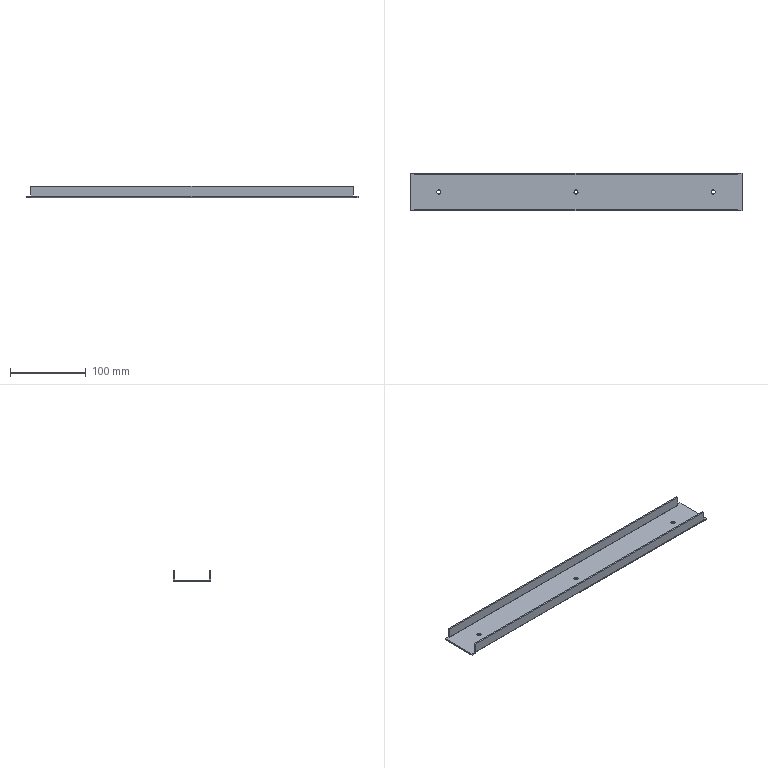Part | STEP file | SX-022-04 | 1 solid | 36 faces | box 438 x 50 x 15 mm | volume 64937 mm3 | plane 26 | cylinder 10 | commonest cylinder face diameters 5.4 x6 0.4 x2 4.4 x2